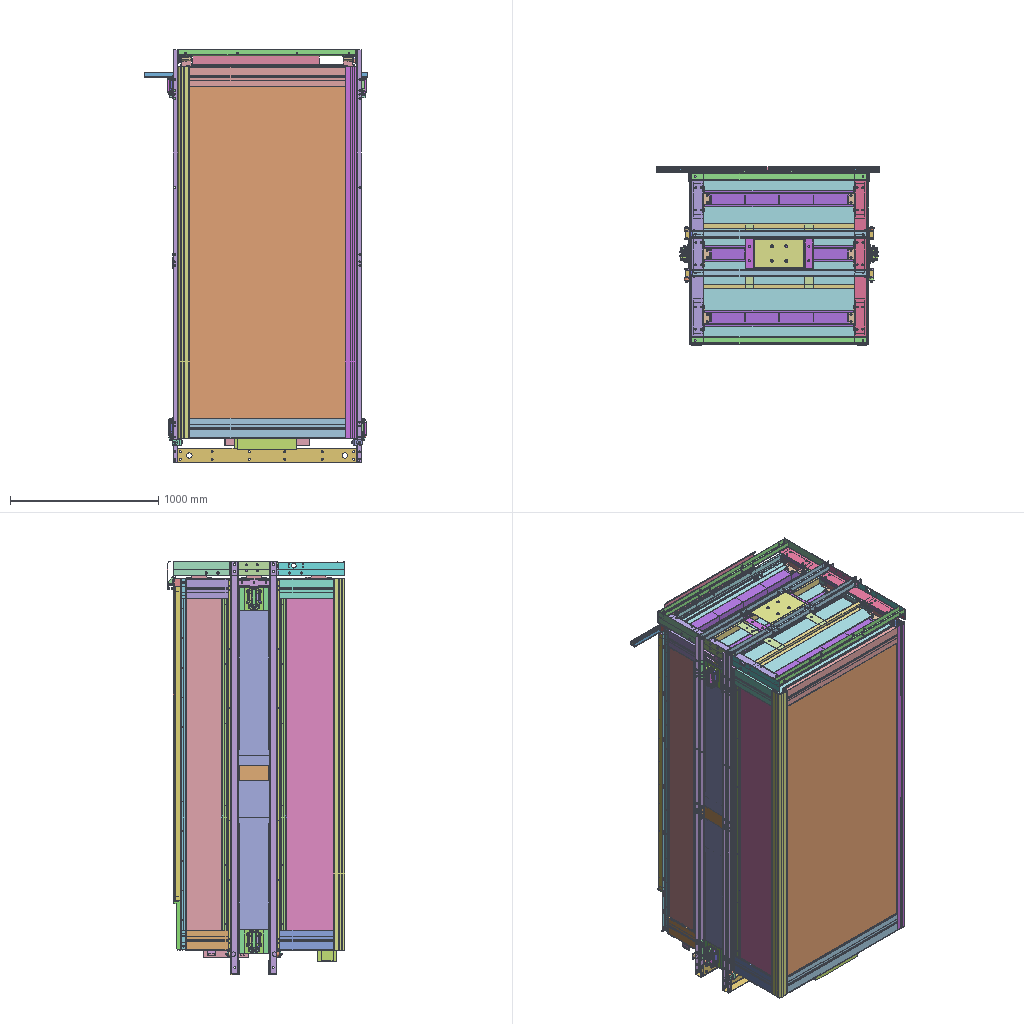Assembly | SolidWorks | 132 different items | 246 placed | box 1500 x 1197 x 2789 mm
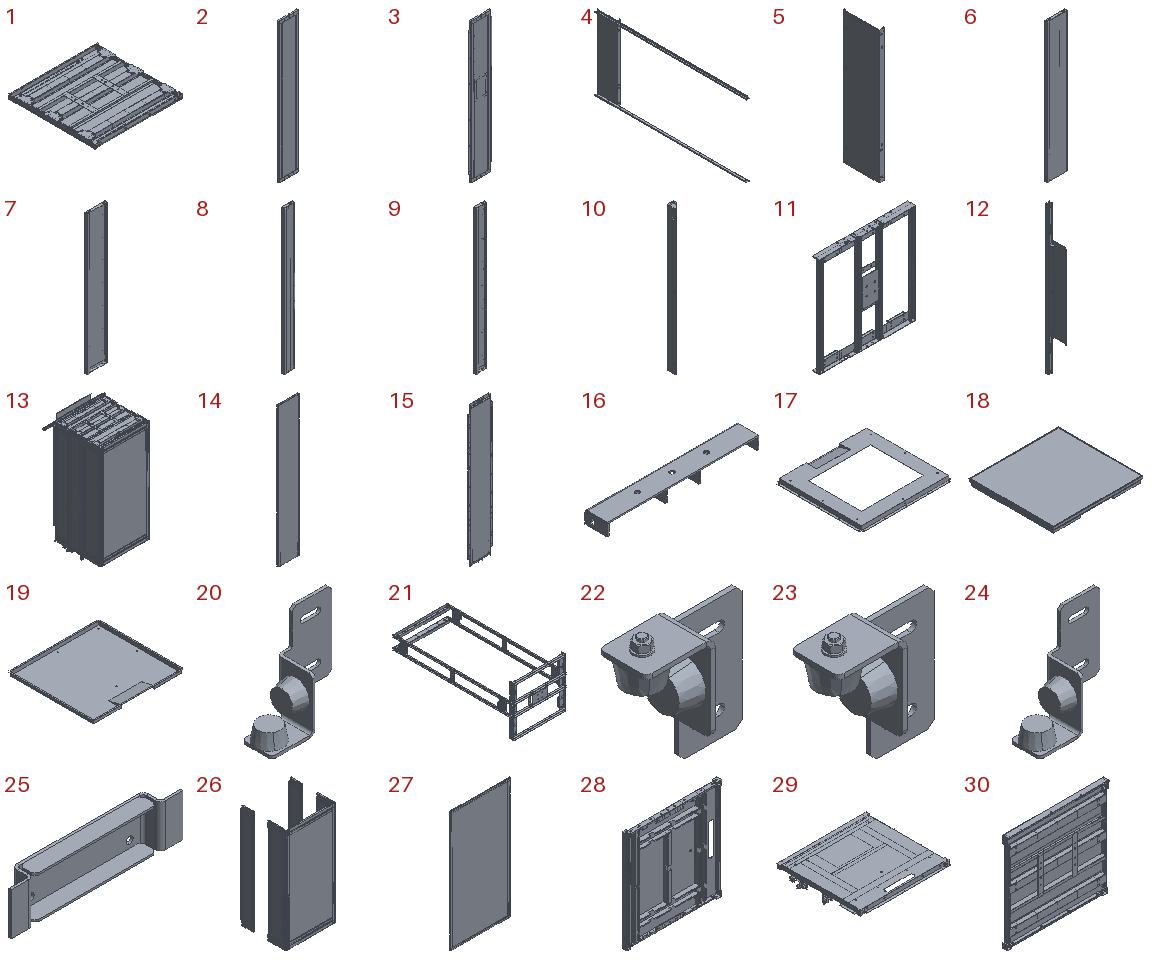Parts list (item | name | quantity | parent item | size | volume | features):
1 | (subassembly) | x1 | in 13 | 1171 x 1143 x 83 mm | 26404069 mm3 | features ReferencePattern 3, MirrorCompFeat 1
2 | (subassembly) | x1 | in 3 | 346 x 32 x 2502 mm | 1579459 mm3 | features MirrorCompFeat 1, ReferencePattern 1
3 | (subassembly) | x1 | in 13 | 424 x 33 x 2502 mm | 3632859 mm3 | -
4 | (subassembly) | x1 | in 13 | 90 x 2502 x 1221 mm | 1703214 mm3 | -
5 | (subassembly) | x1 | in 4 | 50 x 333 x 1221 mm | 642067 mm3 | -
6 | (subassembly) | x1 | in 13 | 310.7 x 50 x 2116 mm | 2074719 mm3 | -
7 | (subassembly) | x1 | in 6 | 310.5 x 50 x 2116 mm | 1201289 mm3 | features MirrorCompFeat 1, ReferencePattern 1
8 | (subassembly) | x1 | in 13 | 160.7 x 50 x 2116 mm | 1348721 mm3 | -
9 | (subassembly) | x1 | in 8 | 160.5 x 50 x 2116 mm | 792691 mm3 | features MirrorCompFeat 1, ReferencePattern 1
10 | (subassembly) | x1 | in 12 | 37 x 51 x 800 mm | 243853 mm3 | features ReferencePattern 2, MirrorCompFeat 1
11 | (subassembly) | x1 | in 21 | 1155 x 95 x 1206 mm | 5315222 mm3 | features ReferencePattern 18, MirrorCompFeat 6, CompositeCurve 1
12 | (subassembly) | x1 | in 13 | 40 x 188.321 x 1500 mm | 981117 mm3 | -
13 | (subassembly) | x1 | - | - | 120553237 mm3 | features InContextFeatHolder 4
14 | (subassembly) | x1 | in 15 | 350 x 30 x 2396 mm | 3626066 mm3 | -
15 | (subassembly) | x1 | - | 428 x 30 x 2502 mm | 4227326 mm3 | -
16 | (subassembly) | x2 | in 15 | 350 x 53 x 30 mm | 92849 mm3 | features ReferencePattern 2, MirrorCompFeat 1
17 | (subassembly) | x1 | - | 1095 x 1035 x 50.189 mm | 845352 mm3 | -
18 | (subassembly) | x1 | in 13 | 1095 x 1035 x 80 mm | 5243599 mm3 | -
19 | (subassembly) | x1 | in 18 | 1095 x 1035 x 45 mm | 1302233 mm3 | -
20 | (subassembly) | x1 | in 29 | 130.5 x 50 x 136 mm | 88035 mm3 | -
21 | (subassembly) | x1 | - | - | 14365446 mm3 | features ReferencePattern 11, MirrorCompFeat 4
22 | (subassembly) | x1 | in 29 | 130.5 x 50 x 136 mm | 88035 mm3 | -
23 | (subassembly) | x1 | in 29 | 130.5 x 50 x 136 mm | 88035 mm3 | -
24 | (subassembly) | x1 | in 29 | 130.5 x 50 x 136 mm | 88035 mm3 | -
25 | (subassembly) | x6 | in 11 | 260 x 30 x 64.5 mm | 102793 mm3 | features MirrorCompFeat 1, ReferencePattern 1
26 | (subassembly) | x1 | in 13 | 1199 x 1107 x 2502 mm | 68599829 mm3 | features ReferencePattern 2, MirrorCompFeat 1
27 | (subassembly) | x1 | in 26 | 1135 x 18 x 2317 mm | 26409670 mm3 | -
28 | (subassembly) | x1 | in 29 | 1093 x 53 x 1171 mm | 3806395 mm3 | features ReferencePattern 2, MirrorCompFeat 1
29 | (subassembly) | x1 | in 13 | 1282 x 1105 x 103.8 mm | 16071700 mm3 | features ReferencePattern 3, InContextFeatHolder 2, MirrorCompFeat 2
30 | (subassembly) | x1 | in 1 | 1171 x 67 x 1143 mm | 7393142 mm3 | features ReferencePattern 9, MirrorCompFeat 3, 3DProfileFeature 1, AEMSimFeature 1
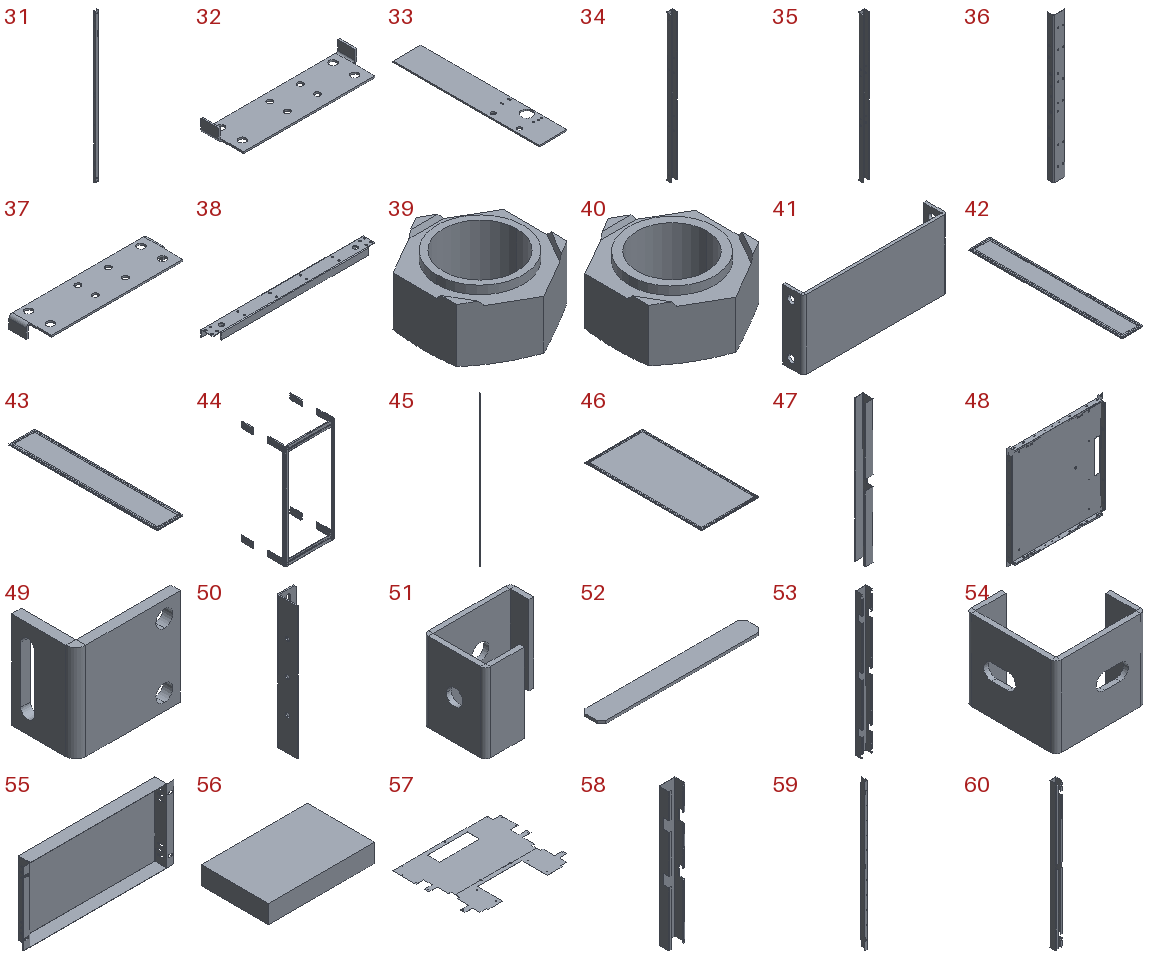31 | - | x4 | in 21 | 50 x 30 x 2775 mm | 844323 mm3 | features ICE 2, FlatPattern 1, SMBaseFlange 1, SheetMetal 1
32 | - | x1 | in 11 | 320 x 90.5 x 30 mm | 114349 mm3 | features ICE 3, FlatPattern 1, SMBaseFlange 1, SheetMetal 1
33 | - | x2 | in 11 | 85 x 445 x 4 mm | 146216 mm3 | features Extrusion 1
34 | - | x2 | in 11 | 50 x 40 x 1190 mm | 552905 mm3 | features ICE 3, FlatPattern 1, SMBaseFlange 1, SheetMetal 1
35 | - | x2 | in 11 | 50 x 40 x 1190 mm | 552403 mm3 | features ICE 3, FlatPattern 1, SMBaseFlange 1, SheetMetal 1
36 | - | x2 | in 11 | 88.5 x 50 x 1155 mm | 598465 mm3 | features ICE 2, Chamfer 1, FlatPattern 1, MoveCopyBody 1, SMBaseFlange 1, SheetMetal 1
37 | - | x1 | in 11 | 320 x 90.5 x 30 mm | 114349 mm3 | features MirrorStock 1
38 | - | x2 | in 21 | 1268 x 100 x 54 mm | 958422 mm3 | features ICE 2, FlatPattern 1, SMBaseFlange 1, SheetMetal 1
39 | - | x8 | in 11 | 24 x 27.713 x 13 mm | 3465 mm3 | features Cut 3, Boss 1, CirPattern 1, Extrusion 1, RefAxis 1
40 | - | x8 | in 11 | 19 x 21.939 x 10 mm | 1791 mm3 | features Cut 3, Boss 1, CirPattern 1, Extrusion 1, RefAxis 1
41 | - | x2 | in 21 | 208 x 30 x 100 mm | 101724 mm3 | features FlatPattern 1, ICE 1, SMBaseFlange 1, SheetMetal 1
42 | - | x2 | in 26 | 313.5 x 2317 x 18 mm | 7344487 mm3 | features ICE 1, WeldMemberFeat 1, WeldmentFeature 1
43 | - | x2 | in 26 | 398.5 x 2317 x 18 mm | 9317148 mm3 | features ICE 1, WeldMemberFeat 1, WeldmentFeature 1
44 | - | x1 | in 26 | 1199 x 1067 x 2502 mm | 8436439 mm3 | features ICE 4, MirrorPattern 2, WeldMemberFeat 2, 3DProfileFeature 1, Cut 1, WeldmentFeature 1
45 | - | x4 | in 26 | 8.5 x 18.686 x 2317 mm | 107612 mm3 | features Extrusion 1
46 | - | x1 | in 27 | 1135 x 2317 x 18 mm | 26409670 mm3 | features ICE 2, WeldMemberFeat 1, WeldmentFeature 1
47 | - | x1 | in 28 | 40 x 51 x 700 mm | 136327 mm3 | features FlatPattern 1, ICE 1, SMBaseFlange 1, SheetMetal 1
48 | - | x1 | in 28 | 1093 x 53 x 1171 mm | 2180191 mm3 | features ICE 12, EdgeFlange 5, Fillet 5, SMBaseFlange 5, Cut 2, Chamfer 1, FlatPattern 1, MirrorPattern 1, SheetMetal 1
49 | - | x1 | in 29 | 65 x 40 x 60 mm | 31981 mm3 | features ICE 2, FlatPattern 1, SMBaseFlange 1, SheetMetal 1
50 | - | x2 | in 28 | 45 x 50 x 319.5 mm | 82672 mm3 | features ICE 3, Chamfer 1, FlatPattern 1, SMBaseFlange 1, SheetMetal 1
51 | - | x2 | in 28 | 56 x 40 x 51 mm | 18577 mm3 | features ICE 2, FlatPattern 1, SMBaseFlange 1, SheetMetal 1
52 | - | x12 | in 25 | 185 x 24 x 3 mm | 13170 mm3 | features Extrusion 1
53 | - | x1 | in 28 | 80 x 51 x 1130 mm | 308482 mm3 | features ICE 3, Chamfer 1, FlatPattern 1, SMBaseFlange 1, SheetMetal 1
54 | - | x2 | in 28 | 56 x 56 x 50 mm | 20650 mm3 | features ICE 4, FlatPattern 1, SMBaseFlange 1, SheetMetal 1
55 | - | x1 | in 29 | 628 x 50 x 305 mm | 273586 mm3 | features EdgeFlange 2, ICE 2, FlatPattern 1, SMBaseFlange 1, SheetMetal 1
56 | - | x1 | in 29 | 465 x 295 x 80 mm | 10974000 mm3 | features Extrusion 1
57 | - | x1 | in 29 | 1195 x 952 x 0.8 mm | 633597 mm3 | features ICE 11, Cut 5, Fillet 2, Extrusion 1
58 | - | x2 | in 28 | 80 x 51 x 687 mm | 188870 mm3 | features ICE 2, FlatPattern 1, SMBaseFlange 1, SheetMetal 1, WeldmentFeature 1
59 | - | x1 | in 28 | 35 x 51.5 x 1130 mm | 184167 mm3 | features ICE 4, Chamfer 1, FlatPattern 1, SMBaseFlange 1, SheetMetal 1
60 | - | x1 | in 28 | 48 x 51 x 1130 mm | 366572 mm3 | features ICE 6, Chamfer 1, FlatPattern 1, SMBaseFlange 1, SheetMetal 1
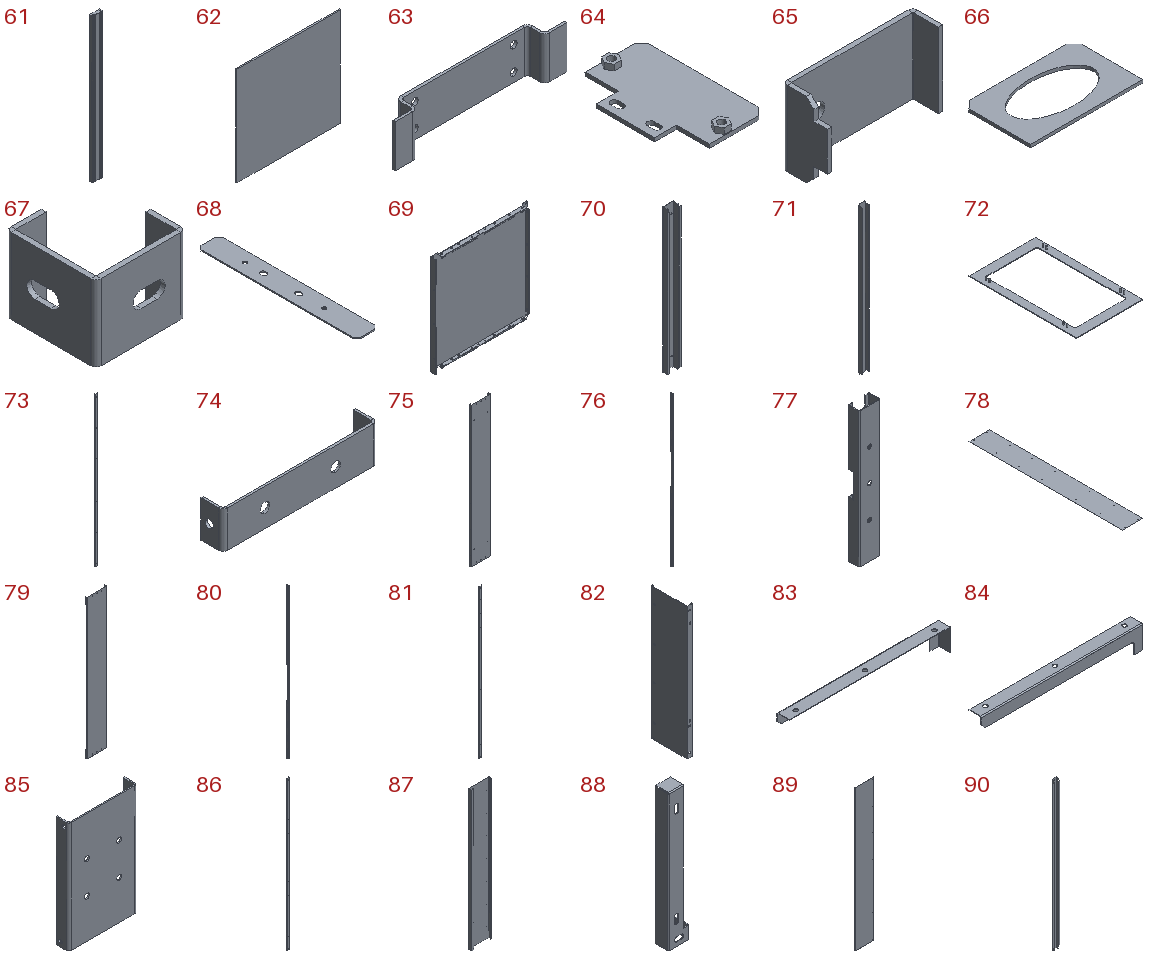61 | - | x1 | in 1 | 50 x 15 x 750 mm | 379215 mm3 | features ICE 3, Fillet 2, Extrusion 1, MirrorSolid 1
62 | - | x1 | in 1 | 1130 x 15 x 1072 mm | 18170400 mm3 | features 3DProfileFeature 1, Extrusion 1, ICE 1
63 | - | x6 | in 25 | 260 x 30 x 64.5 mm | 76453 mm3 | features FlatPattern 1, ICE 1, SMBaseFlange 1, SheetMetal 1
64 | - | x6 | in 1 | 107 x 170 x 13 mm | 76885 mm3 | features ICE 4, Chamfer 1, CombineBodies 1, Extrusion 1
65 | - | x2 | in 30 | 87 x 30 x 50 mm | 18448 mm3 | features ICE 4, Chamfer 1, FlatPattern 1, SMBaseFlange 1, SheetMetal 1
66 | - | x15 | in 30 | 75 x 46 x 2 mm | 4258 mm3 | features Chamfer 1, Cut 1, FlatPattern 1, SMBaseFlange 1, SheetMetal 1
67 | - | x2 | in 30 | 56 x 56 x 47 mm | 19347 mm3 | features ICE 3, FlatPattern 1, SMBaseFlange 1, SheetMetal 1
68 | - | x2 | in 30 | 60 x 437.5 x 3 mm | 76492 mm3 | features ICE 2, Chamfer 1, Cut 1, Extrusion 1
69 | - | x1 | in 30 | 1143 x 67 x 1171 mm | 4628360 mm3 | features ICE 14, EdgeFlange 5, SMBaseFlange 3, Cut 2, Fillet 1, FlatPattern 1, MirrorPattern 1, SheetMetal 1
70 | - | x3 | in 30 | 106 x 50 x 1127 mm | 661257 mm3 | features ICE 3, Chamfer 1, Cut 1, FlatPattern 1, SMBaseFlange 1, SheetMetal 1
71 | - | x2 | in 30 | 50 x 30 x 1127 mm | 233640 mm3 | features Chamfer 1, FlatPattern 1, ICE 1, SMBaseFlange 1, SheetMetal 1
72 | - | x1 | in 3 | 218 x 350 x 12 mm | 54399 mm3 | features ICE 3, Fillet 1, FlatPattern 1, SMBaseFlange 1, SheetMetal 1
73 | - | x2 | in 3 | 39 x 15 x 2234 mm | 228036 mm3 | features ICE 2, FlatPattern 1, SMBaseFlange 1, SheetMetal 1
74 | - | x2 | in 11 | 210 x 30 x 50 mm | 37654 mm3 | features ICE 2, FlatPattern 1, SMBaseFlange 1, SheetMetal 1
75 | - | x1 | in 2 | 346 x 32 x 2502 mm | 1082506 mm3 | features ICE 7, Cut 1, FlatPattern 1, SMBaseFlange 1, SheetMetal 1
76 | - | x1 | in 2 | 33.5 x 28 x 2396 mm | 191583 mm3 | features ICE 6, LPattern 2, EdgeFlange 1, FlatPattern 1, SMBaseFlange 1, SheetMetal 1
77 | - | x2 | in 2 | 53 x 28 x 341 mm | 56893 mm3 | features ICE 2, FlatPattern 1, SMBaseFlange 1, SheetMetal 1
78 | - | x1 | in 3 | 322 x 2394 x 0.8 mm | 615975 mm3 | features Extrusion 1, ICE 1
79 | - | x1 | in 3 | 350 x 30 x 2502 mm | 926955 mm3 | features ICE 3, SMBaseFlange 2, Cut 1, FlatPattern 1, MirrorPattern 1, SheetMetal 1
80 | - | x1 | in 2 | 33.5 x 28 x 2396 mm | 191583 mm3 | features MirrorStock 1
81 | - | x1 | in 4 | 40 x 25 x 2501 mm | 530573 mm3 | features ICE 3, Chamfer 2, Cut 2, FlatPattern 1, SMBaseFlange 1, SheetMetal 1
82 | - | x1 | in 5 | 50 x 333 x 1221 mm | 608956 mm3 | features ICE 8, Cut 4, Chamfer 1, FlatPattern 1, SMBaseFlange 1, SheetMetal 1
83 | - | x1 | in 5 | 330 x 25 x 46.5 mm | 16555 mm3 | features ICE 4, EdgeFlange 2, Chamfer 1, Fillet 1, FlatPattern 1, SMBaseFlange 1, SheetMetal 1
84 | - | x1 | in 5 | 330 x 25 x 46.5 mm | 16555 mm3 | features ICE 4, EdgeFlange 2, Chamfer 1, Fillet 1, FlatPattern 1, SMBaseFlange 1, SheetMetal 1
85 | - | x1 | in 11 | 208 x 38 x 335 mm | 358590 mm3 | features Cut 1, FlatPattern 1, ICE 1, SMBaseFlange 1, SheetMetal 1
86 | - | x1 | in 4 | 40 x 25 x 2501 mm | 530573 mm3 | features MirrorStock 1
87 | - | x1 | in 7 | 310.5 x 50 x 2116 mm | 1139747 mm3 | features ICE 7, EdgeFlange 2, Cut 1, FlatPattern 1, SMBaseFlange 1, SheetMetal 1
88 | - | x1 | in 7 | 47.5 x 30 x 307.5 mm | 30771 mm3 | features ICE 4, EdgeFlange 3, FlatPattern 1, SMBaseFlange 1, SheetMetal 1
89 | - | x1 | in 6 | 278 x 12 x 2116 mm | 610438 mm3 | features ICE 4, FlatPattern 1, SMBaseFlange 1, SheetMetal 1
90 | - | x2 | in 6, 8 | 100 x 30.8 x 2109 mm | 262992 mm3 | features ICE 2, Chamfer 1, FlatPattern 1, MoveCopyBody 1, SMBaseFlange 1, SheetMetal 1
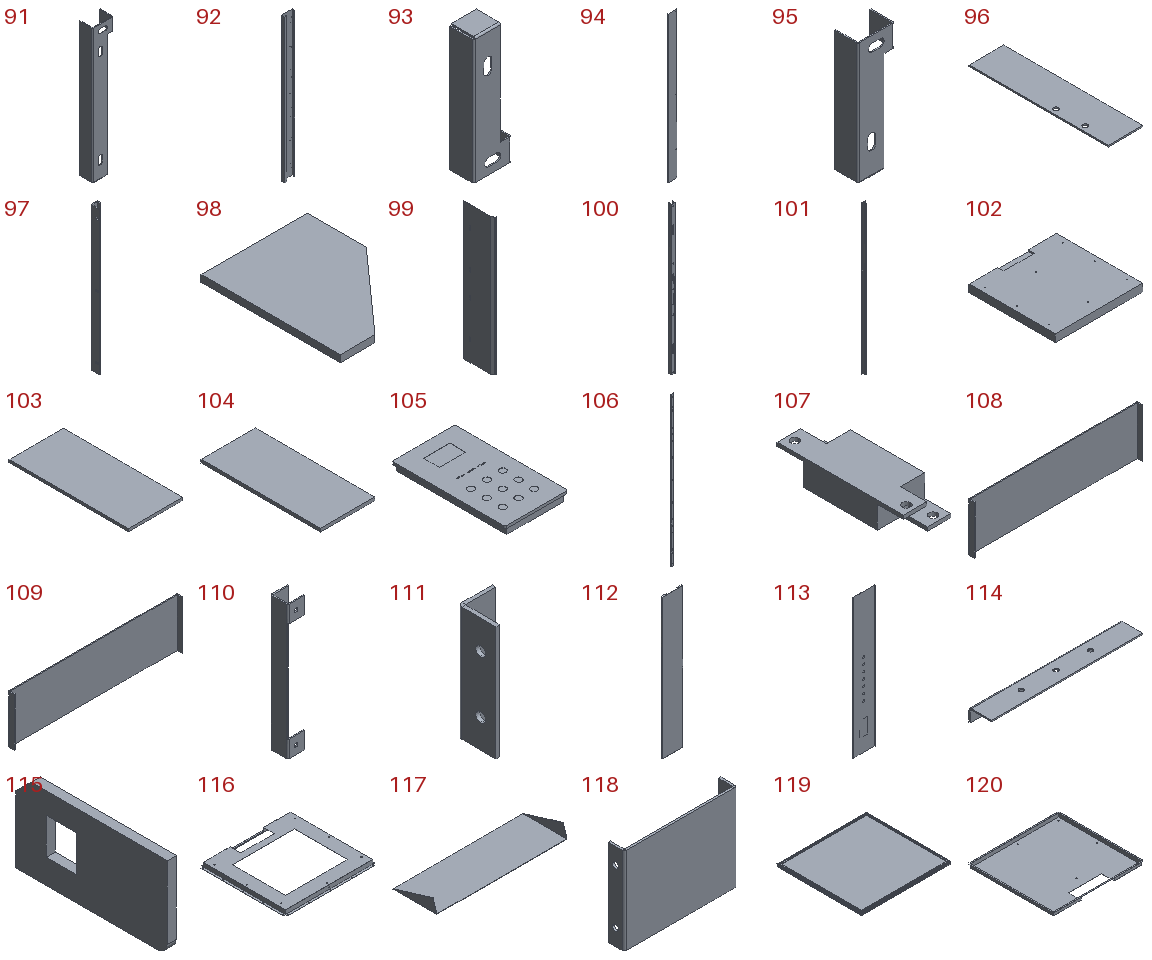91 | - | x1 | in 7 | 47.5 x 30 x 307.5 mm | 30771 mm3 | features MirrorStock 1
92 | - | x1 | in 9 | 160.5 x 50 x 2116 mm | 758867 mm3 | features ICE 7, EdgeFlange 2, Cut 1, FlatPattern 1, SMBaseFlange 1, SheetMetal 1
93 | - | x1 | in 9 | 47 x 30 x 157 mm | 16912 mm3 | features ICE 4, EdgeFlange 3, Cut 1, FlatPattern 1, SMBaseFlange 1, SheetMetal 1
94 | - | x1 | in 8 | 128 x 12 x 2116 mm | 293038 mm3 | features ICE 4, FlatPattern 1, SMBaseFlange 1, SheetMetal 1
95 | - | x1 | in 9 | 47 x 30 x 157 mm | 16912 mm3 | features MirrorStock 1
96 | - | x2 | in 11 | 95 x 380 x 4 mm | 143338 mm3 | features Extrusion 1
97 | - | x1 | in 10 | 37 x 51 x 800 mm | 235979 mm3 | features ICE 3, Cut 1, FlatPattern 1, SMBaseFlange 1, SheetMetal 1
98 | - | x4 | in 10 | 30.5 x 40 x 2 mm | 1968 mm3 | features Extrusion 1
99 | - | x1 | in 12 | 17 x 184.321 x 850 mm | 163173 mm3 | features FlatPattern 1, ICE 1, SMBaseFlange 1, SheetMetal 1
100 | - | x1 | in 12 | 37 x 30 x 1500 mm | 289568 mm3 | features FlatPattern 1, ICE 1, SMBaseFlange 1, SheetMetal 1
101 | - | x1 | in 12 | 40 x 29.5 x 1500 mm | 284523 mm3 | features Cut 1, Extrusion 1, ICE 1
102 | - | x1 | - | 1145 x 1125 x 100 mm | 128094667 mm3 | features ICE 3, Extrusion 1
103 | - | x1 | - | 100 x 220 x 5 mm | 110000 mm3 | features Extrusion 1
104 | - | x1 | - | 100 x 220 x 6 mm | 132000 mm3 | features Extrusion 1
105 | - | x1 | - | 238 x 428 x 35 mm | 3242262 mm3 | features ICE 3, Extrusion 1, MoveCopyBody 1
106 | - | x2 | in 15 | 39 x 12 x 2234 mm | 207782 mm3 | features ICE 3, SMBaseFlange 2, FlatPattern 1, SheetMetal 1
107 | - | x6 | in 21 | 64 x 170 x 35 mm | 244149 mm3 | features ICE 3, Extrusion 1
108 | - | x1 | in 14 | 350 x 12 x 100 mm | 73794 mm3 | features FlatPattern 1, SMBaseFlange 1, SheetMetal 1
109 | - | x1 | in 14 | 350 x 12 x 100 mm | 73794 mm3 | features FlatPattern 1, SMBaseFlange 1, SheetMetal 1
110 | - | x2 | in 14 | 25 x 26 x 198 mm | 18838 mm3 | features ICE 2, FlatPattern 1, SMBaseFlange 1, SheetMetal 1
111 | - | x1 | in 14 | 18 x 20 x 60 mm | 4180 mm3 | features FlatPattern 1, ICE 1, SMBaseFlange 1, SheetMetal 1
112 | - | x1 | in 14 | 350 x 25 x 2396 mm | 1834620 mm3 | features ICE 5, FlatPattern 1, SMBaseFlange 1, SheetMetal 1
113 | - | x1 | in 14 | 350 x 12 x 2194 mm | 1602003 mm3 | features FlatPattern 1, ICE 1, SMBaseFlange 1, SheetMetal 1
114 | - | x2 | in 16 | 350 x 53 x 30 mm | 78262 mm3 | features ICE 3, FlatPattern 1, SMBaseFlange 1, SheetMetal 1
115 | - | x8 | in 16 | 3 x 50 x 27 mm | 3647 mm3 | features Cut 1, Extrusion 1, Fillet 1
116 | - | x1 | - | 1095 x 1035 x 50 mm | 787160 mm3 | features ICE 7, EdgeFlange 2, FlatPattern 1, SMBaseFlange 1, SheetMetal 1
117 | - | x1 | - | 399.001 x 133.5 x 38.5 mm | 58192 mm3 | features EdgeFlange 1, FlatPattern 1, MirrorPattern 1, SMBaseFlange 1, SheetMetal 1
118 | - | x4 | in 21 | 208 x 30 x 160 mm | 163671 mm3 | features FlatPattern 1, ICE 1, SMBaseFlange 1, SheetMetal 1
119 | - | x1 | - | 1095 x 1035 x 30 mm | 24245961 mm3 | features ICE 1, WeldMemberFeat 1, WeldmentFeature 1
120 | - | x1 | in 19 | 1095 x 1035 x 45 mm | 1236124 mm3 | features ICE 4, EdgeFlange 2, FlatPattern 1, SMBaseFlange 1, SheetMetal 1
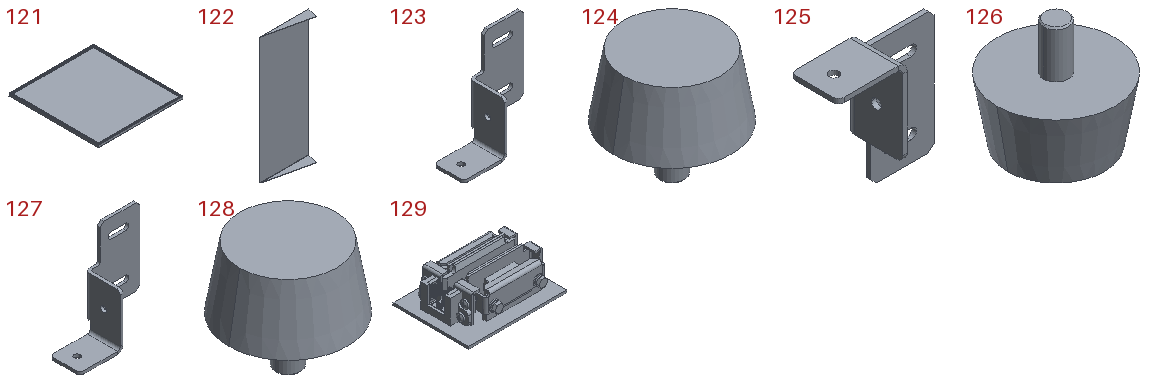121 | - | x1 | in 18 | 1035 x 1095 x 35 mm | 3941366 mm3 | features ICE 1, WeldMemberFeat 1, WeldmentFeature 1
122 | - | x1 | in 19 | 153.5 x 34 x 399 mm | 66108 mm3 | features EdgeFlange 1, FlatPattern 1, MirrorPattern 1, SMBaseFlange 1, SheetMetal 1
123 | - | x1 | in 20 | 129.5 x 50 x 125 mm | 47149 mm3 | features ICE 4, Fillet 2, Chamfer 1, EdgeFlange 1, FlatPattern 1, SMBaseFlange 1, SheetMetal 1
124 | - | x2 | in 20 | 38 x 38 x 35 mm | 19484 mm3 | features Chamfer 2, MoveCopyBody 2, Extrusion 1, ICE 1
125 | - | x2 | in 22, 23 | 129.5 x 50 x 125 mm | 47149 mm3 | features MirrorStock 1
126 | - | x4 | in 22, 23 | 38 x 38 x 35 mm | 19484 mm3 | features MirrorStock 1
127 | - | x1 | in 24 | 129.5 x 50 x 125 mm | 47149 mm3 | features MirrorStock 1
128 | - | x2 | in 24 | 38 x 38 x 35 mm | 19484 mm3 | features MirrorStock 1
129 | - | x4 | in 21 | - | 358287 mm3 | features BaseBody 39, ICE 1, MoveCopyBody 1
130 | hex nuts, style 1-grades ab gb | x1 | - | - | - | -
131 | hexagon weld nuts gb | x1 | - | - | - | -
132 | plain washers--product grade c gb | x1 | - | - | - | -
Mates (type | each side: item.copy, entity, surface, feature):
In the top assembly
Coincident | 11.1 plane | assembly plane | 2 times
Coincident | assembly face | 107.1 face plane 凸台-拉伸1
Coincident | assembly face | 107.2 face plane 凸台-拉伸1
Coincident | 31.1 face plane 基体-法兰1 | assembly face | 2 times
Coincident | assembly plane | assembly plane | 6 times
Coincident | 18.1 plane | assembly plane
Coincident | 64.1 face plane 凸台-减震垫孔 | 107.1 face plane 凸台-拉伸1
Coincident | 79.1 face plane 基体-法兰1 | 105.1 face plane 凸台-拉伸1
Coincident | 105.1 plane | 3.1 plane
DistanceDim | 105.1 plane | 77.1 face plane 基体-法兰1
Coincident | 15.1 plane | assembly plane
Coincident | 48.1 face plane 边线-法兰9 | 114.1 face plane 基体-法兰1
Coincident | 48.1 face plane 边线-法兰16 | 114.1 face plane 基体-法兰1
Coincident | 75.1 face plane 基体-法兰1 | 103.1 face plane 凸台-拉伸1
DistanceDim | 103.1 face plane 凸台-拉伸1 | 76.1 face plane 基体-法兰1
Coincident | 75.1 face plane 基体-法兰1 | 104.1 face plane 凸台-拉伸1
DistanceDim | 104.1 face plane 凸台-拉伸1 | 76.1 face plane 基体-法兰1
DistanceDim | 104.1 face plane 凸台-拉伸1 | 129.1 face plane OX029YZ-2-solid39
DistanceDim | 103.1 face plane 凸台-拉伸1 | 129.2 face plane OX029YZ-2-solid39
In subassembly 13
Coincident | 13.1 face | 13.1 face
Concentric | 13.1 face | 13.1 face
Coincident | 26.1 plane | 13.1 plane | 3 times
Coincident | 3.2 plane | 13.1 plane
Coincident | 44.1 face plane 立柱 侧横档型材(2) | 77.2 face plane 基体-法兰1
Coincident | 44.1 face plane 立柱 侧横档型材(2) | 79.2 face plane 基体-法兰1
DistanceDim | 121.1 face plane 发光背板型材 边框(1) | 46.1 face plane 自定义 玻璃外框(1)
Coincident | 28.1 plane | 13.1 plane | 2 times
Coincident | 55.1 plane | 13.1 plane
Coincident | 57.1 plane | 13.1 plane | 2 times
Coincident | 57.1 face plane 凸台-拉伸1 | 44.1 face plane 立柱 侧横档型材(2)
Coincident | 48.2 face plane 边线-法兰15 | 79.2 face plane 基体-法兰1
Coincident | 48.2 face plane 基体-法兰1 | 120.1 face plane 基体-法兰1
Symmetric | 124.1 face plane 凸台-拉伸1 | 13.1 face | 13.1 plane | 2 times
Coincident | 30.1 plane | 13.1 plane | 2 times
Coincident | 44.1 face plane 立柱 侧横档型材(2) | 69.1 face plane 边线-法兰18
Coincident | 69.1 face plane 基体-法兰1 | 93.1 face plane 基体-法兰1
Coincident | 69.1 face plane 边线-法兰17 | 92.1 face plane 基体-法兰1
DistanceDim | 92.1 face plane 基体-法兰1 | 65.1 face plane 基体-法兰1
Coincident | 69.1 face plane 边线-法兰17 | 100.1 face plane 基体-法兰1
Coincident | 69.1 select_type:25 | 12.1 plane
Coincident | 69.1 face plane 基体-法兰1 | 87.1 face plane 基体-法兰右
Coincident | 69.1 face plane 基体-法兰1 | 12.1 plane
Coincident | 18.2 plane | 13.1 plane
Coincident | 5.1 plane | 13.1 plane
Coincident | 44.1 face plane 立柱 侧横档型材(2) | 82.1 face plane 基体-法兰1
Coincident | 48.2 face plane 边线-法兰16 | 82.1 face plane 基体-法兰1
Coincident | 86.1 face plane | 87.1 face plane 基体-法兰右 | 2 times
Coincident | 44.1 face plane 立柱 侧横档型材(2) | 81.1 face plane 基体-法兰1
Coincident | 48.2 face plane 基体-法兰1 | 13.1 face
DistanceDim | 13.1 face | 46.1 face plane 自定义 玻璃外框(1)
DistanceDim | 13.1 face | 43.1 face plane 自定义 玻璃外框(1)
In subassembly 3
Coincident | 78.1 plane | 3.3 plane
Coincident | 79.3 plane | 3.3 plane
DistanceDim | 73.1 face plane 基体-法兰1 | 79.3 face plane 基体-法兰1
DistanceDim | 73.2 face plane 基体-法兰1 | 79.3 face plane 基体-法兰1
Coincident | 73.2 face plane 基体-法兰1 | 73.1 face plane 基体-法兰1
Coincident | 75.2 plane | 3.3 plane
Coincident | 75.2 face plane 基体-法兰1 | 73.2 face plane 基体-法兰1
Width | 73.2 face plane 基体-法兰1 | 73.2 face plane 基体-法兰1 | 75.2 face plane 基体-法兰1 | 75.2 face plane 基体-法兰1
Coincident | 75.2 face plane 基体-法兰1 | 73.1 face plane 基体-法兰1
Coincident | 75.2 face plane 基体-法兰1 | 79.3 face plane 基体-法兰1 | 2 times
Coincident | 77.3 plane | 3.3 plane
Coincident | 77.4 plane | 3.3 plane
DistanceDim | 77.4 face plane 基体-法兰1 | 78.1 face plane 凸台-拉伸1
Coincident | 76.2 face plane 边线-法兰1 | 78.1 face plane 凸台-拉伸1
Coincident | 75.2 face plane 基体-法兰1 | 72.1 face plane 基体-法兰1
Coincident | 72.1 plane | 3.3 plane
DistanceDim | 72.1 plane | 75.2 face plane 基体-法兰1
In subassembly 2
Coincident | 75.3 face plane 基体-法兰1 | 77.5 face plane 基体-法兰1 | 2 times
Coincident | 75.3 face plane 基体-法兰1 | 77.6 face plane 基体-法兰1 | 2 times
Coincident | 75.3 face plane 基体-法兰1 | 76.3 face plane 基体-法兰1
Coincident | 77.6 face plane 基体-法兰1 | 76.3 face plane 基体-法兰1
Coincident | 77.5 plane | 2.1 plane
Coincident | 77.6 plane | 2.1 plane
DistanceDim | 76.3 face plane 基体-法兰1 | 2.1 plane
In subassembly 1
Coincident | 70.1 face plane 基体-法兰1 | 64.2 face plane 凸台-减震垫孔
Coincident | 30.2 plane | 1.1 plane | 3 times
Parallel | 64.2 plane | 1.1 plane
Symmetric | 64.2 plane | 70.1 face plane 基体-法兰1 | 70.1 face plane 基体-法兰1
Coincident | 70.1 face plane 基体-法兰1 | 64.3 face plane 凸台-减震垫孔
Parallel | 64.3 plane | 1.1 plane
Symmetric | 70.2 face plane 基体-法兰1 | 70.2 face plane 基体-法兰1 | 64.3 plane
Coincident | 70.1 face plane 基体-法兰1 | 64.4 face plane 凸台-减震垫孔
Parallel | 64.4 plane | 1.1 plane
Symmetric | 70.3 face plane 基体-法兰1 | 70.3 face plane 基体-法兰1 | 64.4 plane
DistanceDim | 64.2 face plane 凸台-梁孔 | 69.2 face plane 边线-法兰9
Coincident | 64.2 face plane 凸台-拉伸3 | 64.3 face plane 凸台-拉伸3
Coincident | 64.3 face plane 凸台-拉伸3 | 64.4 face plane 凸台-拉伸3
DistanceDim | 61.1 face plane 凸台-拉伸1 | 69.2 face plane 基体-法兰1
Coincident | 69.2 face plane 边线-法兰17 | 61.1 face plane 凸台-拉伸1
Coincident | 69.2 face plane 切除-踏板 | 61.1 face plane 镜向1
DistanceDim | 62.1 face plane 凸台-拉伸1 | 69.2 face plane 基体-法兰1
Coincident | 62.1 plane | 1.1 plane
DistanceDim | 62.1 face plane 凸台-拉伸1 | 69.2 face plane 边线-法兰13
In subassembly 30
Coincident | 69.3 face plane 基体-法兰1 | 67.1 face plane 基体-法兰1 | 3 times
Coincident | 69.3 face plane 基体-法兰1 | 65.2 face plane 基体-法兰1 | 2 times
Coincident | 69.3 face plane 边线-法兰17 | 65.2 face plane 基体-法兰1
Coincident | 69.3 plane | 30.3 plane | 2 times
Coincident | 69.3 face plane 基体-法兰1 | 30.3 plane
Coincident | 71.1 plane | 30.3 plane
Coincident | 69.3 face plane 基体-法兰1 | 71.1 face plane 基体-法兰1
Coincident | 71.2 plane | 30.3 plane
Coincident | 69.3 face plane 基体-法兰1 | 71.2 face plane 基体-法兰1
Coincident | 68.1 plane | 30.3 plane
DistanceDim | 68.1 plane | 30.3 plane
Coincident | 71.2 face plane 基体-法兰1 | 68.1 face plane 凸台-拉伸1
Coincident | 71.1 face plane 基体-法兰1 | 68.1 face plane 凸台-拉伸1
Coincident | 70.4 plane | 66.1 plane
Coincident | 70.4 face plane 基体-法兰1 | 66.1 face plane 基体-法兰1
Coincident | 70.4 plane | 66.2 plane
Coincident | 70.4 face plane 基体-法兰1 | 66.2 face plane 基体-法兰1
DistanceDim | 70.4 face cylinder 切除-拉伸2 | 66.1 face plane 基体-法兰1
Coincident | 70.4 plane | 66.3 plane
Coincident | 70.4 face plane 基体-法兰1 | 66.3 face plane 基体-法兰1
Coincident | 70.4 plane | 30.3 plane | 2 times
Coincident | 69.3 face plane 基体-法兰1 | 70.4 face plane 基体-法兰1
Coincident | 70.4 face plane 基体-法兰1 | 68.1 face plane 凸台-拉伸1
Symmetric | 70.4 plane | 66.3 face plane 基体-法兰1 | 66.3 face plane 基体-法兰1
Width | 66.3 face plane 基体-法兰1 | 66.1 face plane 基体-法兰1 | 66.2 face plane 基体-法兰1 | 66.2 face plane 基体-法兰1
Coincident | 70.5 plane | 66.4 plane
Coincident | 70.5 face plane 基体-法兰1 | 66.4 face plane 基体-法兰1
Coincident | 70.5 plane | 66.5 plane
Coincident | 70.5 face plane 基体-法兰1 | 66.5 face plane 基体-法兰1
DistanceDim | 70.5 face cylinder 切除-拉伸2 | 66.4 face plane 基体-法兰1
Coincident | 70.5 plane | 66.6 plane
Coincident | 70.5 face plane 基体-法兰1 | 66.6 face plane 基体-法兰1
Coincident | 70.5 plane | 30.3 plane
Coincident | 69.3 face plane 基体-法兰1 | 70.5 face plane 基体-法兰1
DistanceDim | 70.5 plane | 69.3 face plane 边线-法兰17
Symmetric | 70.5 plane | 66.6 face plane 基体-法兰1 | 66.6 face plane 基体-法兰1
Width | 66.6 face plane 基体-法兰1 | 66.4 face plane 基体-法兰1 | 66.5 face plane 基体-法兰1 | 66.5 face plane 基体-法兰1
Coincident | 70.6 plane | 66.7 plane
Coincident | 70.6 face plane 基体-法兰1 | 66.7 face plane 基体-法兰1
Coincident | 70.6 plane | 66.8 plane
Coincident | 70.6 face plane 基体-法兰1 | 66.8 face plane 基体-法兰1
DistanceDim | 70.6 face cylinder 切除-拉伸2 | 66.7 face plane 基体-法兰1
Coincident | 70.6 plane | 66.9 plane
Coincident | 70.6 face plane 基体-法兰1 | 66.9 face plane 基体-法兰1
Coincident | 70.6 plane | 30.3 plane
Coincident | 69.3 face plane 基体-法兰1 | 70.6 face plane 基体-法兰1
DistanceDim | 70.6 plane | 69.3 face plane 边线-法兰13
Symmetric | 70.6 plane | 66.9 face plane 基体-法兰1 | 66.9 face plane 基体-法兰1
Width | 66.9 face plane 基体-法兰1 | 66.7 face plane 基体-法兰1 | 66.8 face plane 基体-法兰1 | 66.8 face plane 基体-法兰1
In subassembly 18
Coincident | 18.3 face | 18.3 face
Concentric | 18.3 face | 18.3 face
Coincident | 19.1 plane | 18.3 plane | 2 times
Coincident | 120.2 face plane 基体-法兰1 | 18.3 plane
Coincident | 121.2 plane | 18.3 plane | 2 times
Coincident | 120.2 face plane 边线-法兰2 | 121.2 face plane 发光背板型材 边框(1)
In subassembly 19
Coincident | 19.2 face | 19.2 face
Concentric | 19.2 face | 19.2 face
Coincident | 120.3 plane | 19.2 plane | 2 times
Coincident | 120.3 face plane 基体-法兰1 | 19.2 plane
Coincident | 122.1 plane | 19.2 plane
Coincident | 120.3 face plane 基体-法兰1 | 122.1 edge
Coincident | 120.3 face plane 切除-拉伸4 | 122.1 edge | 2 times
In subassembly 12
Coincident | 12.2 face | 12.2 face
Concentric | 12.2 face | 12.2 face
Coincident | 10.1 plane | 12.2 plane | 2 times
Coincident | 97.1 face plane 基体-法兰1 | 100.2 face plane 基体-法兰1 | 2 times
Coincident | 10.1 plane | 100.2 plane
Coincident | 99.1 face plane 基体-法兰1 | 100.2 face plane 基体-法兰1
Coincident | 100.2 face plane 基体-法兰1 | 101.1 face plane 凸台-拉伸1 | 2 times
Coincident | 99.1 plane | 12.2 plane
Coincident | 99.1 face plane 基体-法兰1 | 101.1 face plane 凸台-拉伸1
Coincident | 101.1 plane | 12.2 plane
DistanceDim | 12.2 plane | 101.1 face plane 凸台-拉伸1
In subassembly 10
Coincident | 97.2 face plane 基体-法兰1 | 98.1 face plane 凸台-拉伸1 | 2 times
DistanceDim | 98.1 face plane 凸台-拉伸1 | 97.2 face plane 基体-法兰1
Coincident | 97.2 face plane 基体-法兰1 | 98.2 face plane 凸台-拉伸1 | 2 times
DistanceDim | 98.2 face plane 凸台-拉伸1 | 97.2 face plane 基体-法兰1
Coincident | 97.2 plane | 10.2 plane
Coincident | 97.2 face plane 基体-法兰1 | 10.2 plane | 2 times
In subassembly 26
Coincident | 26.2 face | 26.2 face
Concentric | 26.2 face | 26.2 face
Coincident | 44.2 plane | 26.2 plane | 3 times
Coincident | 44.2 face plane 立柱 侧横档型材(2) | 43.2 face plane 自定义 玻璃外框(1) | 3 times
Coincident | 44.2 face plane 立柱 侧横档型材(2) | 42.1 face plane 自定义 玻璃外框(1) | 2 times
DistanceDim | 44.2 face plane 切除-中心 | 42.1 face plane 自定义 玻璃外框(1)
Coincident | 43.2 face plane 自定义 玻璃外框(1) | 45.1 face plane 凸台-拉伸1 | 2 times
DistanceDim | 43.2 face plane 自定义 玻璃外框(1) | 45.1 face plane 凸台-拉伸1
Coincident | 43.2 face plane 自定义 玻璃外框(1) | 45.2 face plane 凸台-拉伸1
DistanceDim | 45.2 face plane 凸台-拉伸1 | 42.1 face plane 自定义 玻璃外框(1)
Coincident | 45.1 face plane 凸台-拉伸1 | 45.2 face plane 凸台-拉伸1
Coincident | 45.1 face plane 凸台-拉伸1 | 45.3 face plane 凸台-拉伸1 | 2 times
Coincident | 45.2 face plane 凸台-拉伸1 | 45.4 face plane 凸台-拉伸1
Coincident | 45.3 face plane 凸台-拉伸1 | 45.4 face plane 凸台-拉伸1 | 2 times
Coincident | 44.2 face plane 立柱 侧横档型材(2) | 45.3 face plane 凸台-拉伸1
Coincident | 44.2 face plane 立柱 侧横档型材(2) | 46.2 face plane 自定义 玻璃外框(1) | 2 times
Coincident | 44.2 face plane 立柱 后立柱型材(1) | 46.2 edge
Coincident | 46.2 plane | 26.2 plane
In subassembly 27
Coincident | 46.3 plane | 27.1 plane | 2 times
Coincident | 46.3 face plane 自定义 玻璃外框(1) | 27.1 plane
In subassembly 29
Coincident | 50.1 face plane 基体-法兰1 | 123.1 face plane 基体-法兰2
Coincident | 57.2 face plane 凸台-拉伸1 | 55.2 face plane 边线-法兰2
Coincident | 57.2 face plane 切除-盖板前端 | 55.2 face plane 边线-法兰1
Coincident | 28.2 plane | 29.1 plane | 3 times
Coincident | 48.3 face plane 边线-法兰16 | 57.2 face plane 凸台-拉伸1
Coincident | 57.2 plane | 29.1 plane | 2 times
Coincident | 55.2 plane | 29.1 plane
Coincident | 48.3 face plane 边线-法兰16 | 49.1 face plane 基体-法兰1
Concentric | 48.3 face cylinder 薄片4 | 49.1 face cylinder 切除-拉伸2
Parallel | 48.3 face plane 薄片4 | 49.1 face plane 基体-法兰1
DistanceDim | 124.2 face plane 凸台-拉伸1 | 29.1 plane
DistanceDim | 124.3 face plane 凸台-拉伸1 | 48.3 face plane 边线-法兰15
Coincident | 48.3 face plane 基体-法兰1 | 56.1 face plane 凸台-拉伸1
DistanceDim | 56.1 face plane 凸台-拉伸1 | 60.1 face plane 基体-法兰1
Coincident | 56.1 plane | 29.1 plane
In subassembly 22
Concentric | 125.1 face cylinder | 126.1 face cylinder
Coincident | 125.1 face plane | 126.1 face plane
Concentric | 125.1 face cylinder | 126.2 face cylinder
Coincident | 125.1 face plane | 126.2 face plane
In subassembly 24
Concentric | 127.1 face cylinder | 128.1 face cylinder
Coincident | 127.1 face plane | 128.1 face plane
Concentric | 127.1 face cylinder | 128.2 face cylinder
Coincident | 127.1 face plane | 128.2 face plane
In subassembly 23
Concentric | 125.1 face cylinder | 126.1 face cylinder
Coincident | 125.1 face plane | 126.1 face plane
Concentric | 125.1 face cylinder | 126.2 face cylinder
Coincident | 125.1 face plane | 126.2 face plane
In subassembly 28
Coincident | 28.3 face | 28.3 face
Concentric | 28.3 face | 28.3 face
Coincident | 48.4 plane | 28.3 plane | 3 times
Coincident | 48.4 face plane 边线-法兰15 | 50.2 face plane 基体-法兰1
Coincident | 50.2 plane | 28.3 plane
Coincident | 48.4 face plane 边线-法兰16 | 50.2 face plane 基体-法兰1
Coincident | 48.4 face plane 基体-法兰1 | 54.1 face plane 基体-法兰1 | 3 times
Coincident | 48.4 face plane 基体-法兰1 | 51.1 face plane 基体-法兰1 | 3 times
Coincident | 48.4 face plane 基体-法兰1 | 59.1 face plane 基体-法兰1
Coincident | 59.1 plane | 28.3 plane
DistanceDim | 48.4 face plane 边线-法兰11 | 59.1 face plane 基体-法兰1
Coincident | 53.1 plane | 28.3 plane
Coincident | 48.4 face plane 基体-法兰1 | 53.1 face plane 基体-法兰1
DistanceDim | 53.1 face plane 基体-法兰1 | 48.4 face plane 边线-法兰13
Coincident | 48.4 face plane 基体-法兰1 | 58.1 face plane 基体-法兰1
DistanceDim | 58.1 face plane 基体-法兰1 | 48.4 face plane 边线-法兰15
Coincident | 47.1 plane | 28.3 plane
Coincident | 48.4 face plane 基体-法兰1 | 47.1 face plane 基体-法兰1
Coincident | 60.2 plane | 28.3 plane
Coincident | 48.4 face plane 基体-法兰1 | 60.2 face plane 基体-法兰1
DistanceDim | 60.2 face plane 基体-法兰1 | 48.4 face plane 边线-法兰11
Coincident | 58.1 face plane 基体-法兰1 | 60.2 face plane 基体-法兰1
Coincident | 48.4 face plane 基体-法兰1 | 51.2 face plane 基体-法兰1 | 2 times
Coincident | 48.4 face plane 边线-法兰11 | 51.2 face plane 基体-法兰1
Coincident | 48.4 face plane 基体-法兰1 | 54.2 face plane 基体-法兰1 | 3 times
Coincident | 58.1 face plane 切除-拉伸1 | 47.1 face plane 基体-法兰1
In subassembly 20
Concentric | 123.2 face cylinder 切除-拉伸4 | 124.4 face cylinder 凸台-拉伸2
Coincident | 123.2 face plane 基体-法兰2 | 124.4 face plane 凸台-拉伸1
Concentric | 123.2 face cylinder 切除-拉伸5 | 124.5 face cylinder 凸台-拉伸2
Coincident | 123.2 face plane 边线-法兰3 | 124.5 face plane 凸台-拉伸1
In subassembly 4
Coordinate | 5.2 select_type:25 | 4.1 select_type:11
Coincident | 82.2 face plane 基体-法兰1 | 81.2 face plane 基体-法兰1 | 2 times
DistanceDim | 81.2 face plane 基体-法兰1 | 82.2 face plane 基体-法兰1
Coincident | 86.2 face plane | 81.2 face plane 基体-法兰1 | 2 times
Coincident | 82.2 face plane 基体-法兰1 | 86.2 face plane
In subassembly 5
Coincident | 82.3 plane | 5.3 plane
Coincident | 82.3 face plane 基体-法兰1 | 5.3 plane | 2 times
Coincident | 82.3 face plane 基体-法兰1 | 84.1 face plane 边线-法兰1 | 2 times
Coincident | 82.3 face plane 基体-法兰1 | 84.1 face plane 边线-法兰2
Coincident | 82.3 face plane 基体-法兰1 | 83.1 face plane 边线-法兰1 | 2 times
Coincident | 82.3 face plane 基体-法兰1 | 83.1 face plane 边线-法兰2
In subassembly 8
Coincident | 8.1 face | 8.1 face
Concentric | 8.1 face | 8.1 face
Coincident | 9.1 plane | 8.1 plane | 3 times
DistanceDim | 94.1 plane | 92.2 face plane 基体-法兰1 | 2 times
Coincident | 92.2 face plane 基体-法兰1 | 94.1 face plane 基体-法兰1
Coincident | 90.1 plane | 8.1 plane
Coincident | 92.2 face plane 基体-法兰1 | 90.1 face plane 基体-法兰1
DistanceDim | 90.1 face plane 基体-法兰1 | 92.2 face plane 基体-法兰1
In subassembly 9
Coincident | 92.3 face plane 基体-法兰1 | 93.2 face plane 基体-法兰1 | 2 times
Coincident | 92.3 face plane 基体-法兰1 | 93.2 face plane 边线-法兰2
Coincident | 92.3 plane | 9.2 plane | 3 times
In subassembly 6
Coincident | 6.1 face | 6.1 face
Concentric | 6.1 face | 6.1 face
Coincident | 7.1 plane | 6.1 plane | 3 times
Symmetric | 87.2 face plane 基体-法兰右 | 87.2 face plane 基体-法兰右 | 90.2 plane
Coincident | 87.2 face plane 基体-法兰右 | 90.2 plane
DistanceDim | 89.1 plane | 87.2 face plane 基体-法兰右 | 2 times
Coincident | 89.1 plane | 6.1 plane
DistanceDim | 90.2 face plane 基体-法兰1 | 87.2 face plane 基体-法兰右
In subassembly 7
Coincident | 87.3 face plane 基体-法兰右 | 88.1 face plane 基体-法兰1 | 2 times
Coincident | 87.3 face plane 基体-法兰右 | 88.1 face plane 边线-法兰2
Coincident | 87.3 plane | 7.2 plane | 3 times
In subassembly 15
Coincident | 16.1 plane | 15.2 plane
Coincident | 114.2 face plane 基体-法兰1 | 114.3 face plane 基体-法兰1
Coincident | 16.2 plane | 15.2 plane
Coincident | 112.1 face plane 基体-法兰1 | 106.1 face plane 基体-法兰1
Coincident | 112.1 face plane 基体-法兰1 | 106.2 face plane 基体-法兰1
Symmetric | 112.1 face plane 基体-法兰1 | 112.1 face plane 基体-法兰1 | 15.2 plane | 2 times
Width | 112.1 face plane 基体-法兰1 | 112.1 face plane 基体-法兰1 | 106.1 face plane 基体-法兰1 | 106.1 face plane 基体-法兰1
Width | 112.1 face plane 基体-法兰1 | 112.1 face plane 基体-法兰1 | 106.2 face plane 基体-法兰1 | 106.2 face plane 基体-法兰1
Coincident | 112.1 face plane 基体-法兰1 | 114.2 face plane 基体-法兰1
Coincident | 112.1 face plane 基体-法兰1 | 114.3 face plane 基体-法兰1
Coincident | 108.1 face plane 基体-法兰1 | 114.2 face plane 基体-法兰1
DistanceDim | 106.1 face plane 基体-法兰1 | 113.1 face plane 基体-法兰1
DistanceDim | 106.2 face plane 基体-法兰1 | 113.1 face plane 基体-法兰1
Coincident | 108.1 face plane 基体-法兰1 | 15.2 plane
Coincident | 113.1 face plane 基体-法兰1 | 15.2 plane
In subassembly 14
Coincident | 112.2 face plane 基体-法兰1 | 108.2 face plane 基体-法兰1 | 2 times
Coincident | 112.2 face plane 基体-法兰1 | 113.2 face plane 基体-法兰1
DistanceDim | 113.2 face plane 基体-法兰1 | 112.2 face plane 基体-法兰1
Coincident | 112.2 face plane 基体-法兰1 | 110.1 face plane 基体-法兰1 | 3 times
Coincident | 112.2 face plane 基体-法兰1 | 110.2 face plane 基体-法兰1 | 3 times
Coincident | 112.2 face plane 基体-法兰1 | 111.1 face plane 基体-法兰1 | 2 times
Coincident | 112.2 face plane 基体-法兰1 | 109.1 face plane 基体-法兰1 | 2 times
DistanceDim | 112.2 face plane 基体-法兰1 | 108.2 face plane 基体-法兰1
Coincident | 108.2 face plane 基体-法兰1 | 113.2 face plane 基体-法兰1
Coincident | 113.2 face plane 基体-法兰1 | 109.1 face plane 基体-法兰1
DistanceDim | 111.1 face plane 基体-法兰1 | 109.1 face plane 基体-法兰1
In subassembly 16
Coordinate | 114.4 select_type:25 | 16.3 select_type:11
Coincident | 114.4 face plane 基体-法兰1 | 115.1 face plane 凸台-拉伸1 | 3 times
Coincident | 114.4 face plane 基体-法兰1 | 115.2 face plane 凸台-拉伸1 | 2 times
DistanceDim | 115.2 face plane 凸台-拉伸1 | 115.3 face plane 凸台-拉伸1
In subassembly 21
Coincident | 38.1 plane | 21.1 plane
Coincident | 38.1 face plane 基体-法兰1 | 21.1 plane
DistanceDim | 31.2 face plane 基体-法兰1 | 38.1 face plane 基体-法兰1
Coincident | 38.1 face plane 基体-法兰1 | 31.2 face plane 基体-法兰1 | 2 times
Coincident | 118.1 plane | 21.1 plane
DistanceDim | 118.1 face plane 基体-法兰1 | 31.2 face plane 基体-法兰1
DistanceDim | 31.2 face plane 基体-法兰1 | 118.1 face plane 基体-法兰1
Coincident | 118.1 face plane 基体-法兰1 | 129.3 face plane OX029YZ-2-solid39 | 2 times
Coincident | 129.3 plane | 21.1 plane
Coincident | 41.1 plane | 21.1 plane
DistanceDim | 41.1 face plane 基体-法兰1 | 31.2 face plane 基体-法兰1
Coincident | 118.2 plane | 21.1 plane
DistanceDim | 31.2 face plane 基体-法兰1 | 118.2 face plane 基体-法兰1
DistanceDim | 118.2 face plane 基体-法兰1 | 31.2 face plane 基体-法兰1
Coincident | 129.4 plane | 21.1 plane
Coincident | 118.2 face plane 基体-法兰1 | 129.4 face plane OX029YZ-2-solid39 | 2 times
Coincident | 11.2 plane | 21.1 plane | 2 times
DistanceDim | 31.2 face plane 基体-法兰1 | 41.1 face plane 基体-法兰1
Coincident | 31.2 face plane 基体-法兰1 | 31.3 face plane 基体-法兰1 | 3 times
Coincident | 38.2 face plane 基体-法兰1 | 31.3 face plane 基体-法兰1
DistanceDim | 38.1 face plane 基体-法兰1 | 38.2 face plane 基体-法兰1
Coincident | 31.2 face plane 基体-法兰1 | 32.1 face plane 基体-法兰1
Coincident | 63.1 face plane 基体-法兰1 | 107.3 face plane 凸台-拉伸1
Width | 63.1 face plane 基体-法兰1 | 63.1 face plane 基体-法兰1 | 107.3 face plane 切除-拉伸1 | 107.3 face plane 切除-拉伸1
Coincident | 63.1 face plane 基体-法兰1 | 107.4 face plane 凸台-拉伸1
Width | 63.2 face plane 基体-法兰1 | 63.2 face plane 基体-法兰1 | 107.4 face plane 切除-拉伸1 | 107.4 face plane 切除-拉伸1
Coincident | 63.1 face plane 基体-法兰1 | 107.5 face plane 凸台-拉伸1
Width | 63.3 face plane 基体-法兰1 | 63.3 face plane 基体-法兰1 | 107.5 face plane 切除-拉伸1 | 107.5 face plane 切除-拉伸1
Concentric | 63.1 face cylinder 切除-拉伸1 | 107.3 face cylinder 切除-拉伸3
Concentric | 63.2 face cylinder 切除-拉伸1 | 107.4 face cylinder 切除-拉伸3
Concentric | 63.3 face cylinder 切除-拉伸1 | 107.5 face cylinder 切除-拉伸3
In subassembly 11
Coincident | 34.1 plane | 11.3 plane
Coincident | 36.1 face plane 基体-法兰1 | 11.3 plane
DistanceDim | 36.1 face plane 基体-法兰1 | 36.2 face plane 基体-法兰1
Coincident | 34.1 face plane 基体-法兰1 | 36.1 face plane 基体-法兰1
Coincident | 36.1 plane | 11.3 plane
Coincident | 35.1 plane | 11.3 plane
Coincident | 36.1 face plane 基体-法兰1 | 35.1 face plane 基体-法兰1
Coincident | 35.2 plane | 11.3 plane
Coincident | 36.1 face plane 基体-法兰1 | 35.2 face plane 基体-法兰1
DistanceDim | 35.2 plane | 11.3 plane
Coincident | 34.2 plane | 11.3 plane
Coincident | 36.1 face plane 基体-法兰1 | 34.2 face plane 基体-法兰1 | 2 times
Coincident | 85.1 plane | 11.3 plane | 2 times
Coincident | 74.1 plane | 11.3 plane
Concentric | 35.2 face cylinder 切除-拉伸2 | 74.1 face cylinder 切除-拉伸2
Parallel | 35.2 face plane 基体-法兰1 | 74.1 face plane 基体-法兰1
Concentric | 36.1 face cylinder 切除-拉伸1 | 40.1 face cylinder 拉伸1
Coincident | 36.1 face plane 基体-法兰1 | 40.1 face plane 拉伸2
Coincident | 36.1 face plane 基体-法兰1 | 39.1 face plane 拉伸2
Concentric | 36.1 face cylinder 切除-拉伸1 | 39.1 face cylinder 拉伸1
Coincident | 36.1 face plane 基体-法兰1 | 96.1 face plane 凸台-拉伸2 | 3 times
Coincident | 32.2 plane | 11.3 plane
Coincident | 36.1 face plane 基体-法兰1 | 32.2 face plane 基体-法兰1 | 2 times
Coincident | 36.1 face plane 基体-法兰1 | 40.2 face plane 拉伸2
Concentric | 36.1 face cylinder 切除-拉伸1 | 40.2 face cylinder 拉伸1
Coincident | 36.1 face plane 基体-法兰1 | 40.3 face plane 拉伸2
Concentric | 36.1 face cylinder 切除-拉伸1 | 40.3 face cylinder 拉伸1
Coincident | 36.1 face plane 基体-法兰1 | 40.4 face plane 拉伸2
Concentric | 36.1 face cylinder 切除-拉伸1 | 40.4 face cylinder 拉伸1
Coincident | 36.1 face plane 基体-法兰1 | 39.2 face plane 拉伸2
Concentric | 36.1 face cylinder 切除-拉伸1 | 39.2 face cylinder 拉伸1
Coincident | 39.3 edge | 32.2 face plane 基体-法兰1
Concentric | 32.2 face cylinder 切除-拉伸2 | 39.3 face cylinder 拉伸1
Concentric | 32.2 face cylinder 切除-拉伸2 | 39.4 face cylinder 拉伸1
Coincident | 36.1 face plane 基体-法兰1 | 33.1 face plane 凸台-拉伸2 | 3 times
Coincident | 36.1 face plane 基体-法兰1 | 63.4 face plane 基体-法兰1
Coincident | 36.1 face plane 基体-法兰1 | 63.5 face plane 基体-法兰1
Coincident | 36.1 face plane 基体-法兰1 | 63.6 face plane 基体-法兰1
Coincident | 39.4 face plane 拉伸2 | 32.2 face plane 基体-法兰1
Coincident | 63.4 face plane 基体-法兰1 | 63.6 face plane 基体-法兰1
Coincident | 36.1 face plane 基体-法兰1 | 34.1 face plane 基体-法兰1
DistanceDim | 35.1 plane | 11.3 plane
DistanceDim | 85.1 face plane 基体-法兰1 | 35.2 face plane 基体-法兰1
Concentric | 36.1 face cylinder 切除-拉伸2 | 63.5 face cylinder 切除-拉伸1
Parallel | 36.1 face plane 基体-法兰1 | 52.1 face plane 凸台-拉伸1
Concentric | 36.1 face cylinder 切除-拉伸2 | 63.4 face cylinder 切除-拉伸1
Concentric | 36.1 face cylinder 切除-拉伸2 | 63.6 face cylinder 切除-拉伸1
In subassembly 25
Coincident | 52.2 plane | 25.1 plane
Coincident | 63.7 face plane 基体-法兰1 | 52.2 face plane 凸台-拉伸1 | 2 times